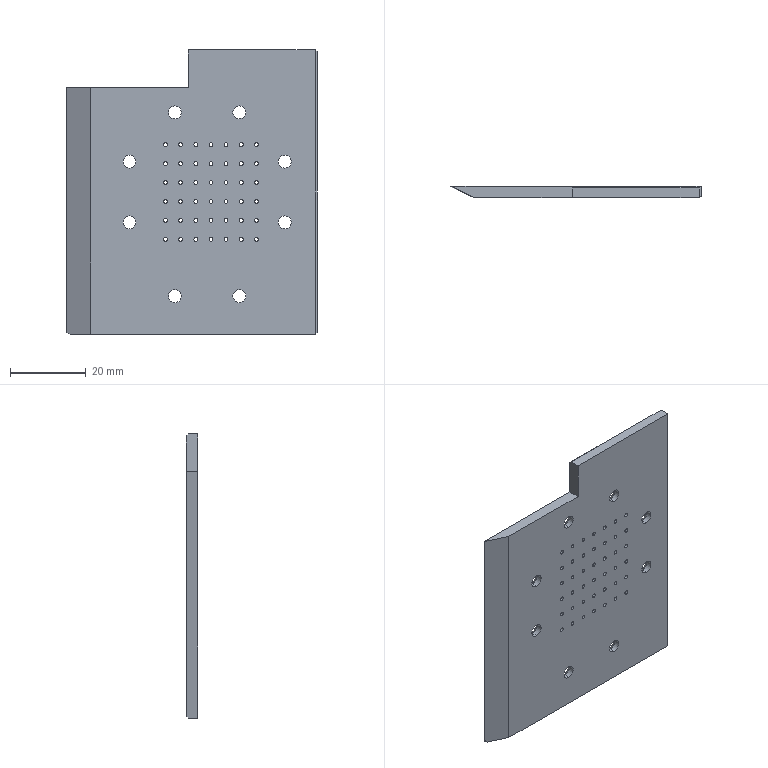Part | STEP file | 10000020503swp000-1 | 1 solid | 130 faces | box 66 x 3 x 75 mm | volume 12831 mm3 | cylinder 100 | cone 16 | plane 14 | commonest cylinder face diameters 1 x84 3.4 x16